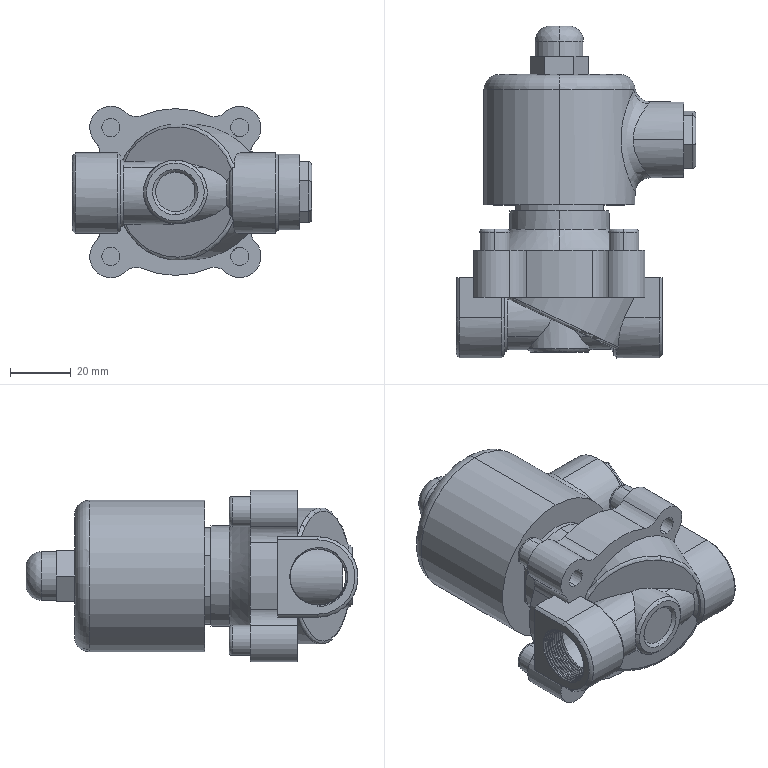Part | SolidWorks | 10 solids | 311 faces | box 79 x 109.5 x 56.5 mm | volume 176709 mm3 | cylinder 155 | plane 98 | spline 46 | torus 12 | commonest cylinder face diameters 19.583 x40 18.5 x37 45 x17 10 x16 6 x8 2 x6